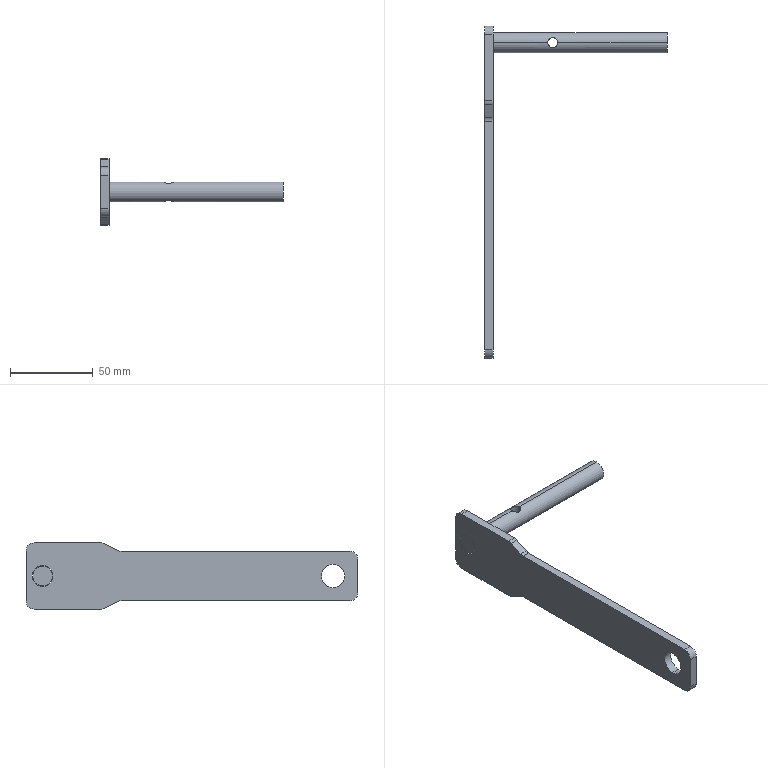Part | SolidWorks | features ICE 2, Fillet 1, Sweep 1 | 2 solids | 28 faces | box 110 x 200 x 40 mm | volume 43181 mm3 | cylinder 16 | plane 12 | commonest cylinder face diameters 10 x8 6 x2 12 x2 12.5 x2 14 x2
STEP:
#1=CARTESIAN_POINT('',(154.,-190.,-6.));
#2=VERTEX_POINT('',#1);
#3=CARTESIAN_POINT('',(148.,-190.,-6.));
#4=VERTEX_POINT('',#3);
#5=CARTESIAN_POINT('',(154.,-190.,-6.));
#6=CARTESIAN_POINT('',(154.,-190.199,-6.));
#7=CARTESIAN_POINT('',(153.98,-190.401,-5.99));
#8=CARTESIAN_POINT('',(153.901,-190.79,-5.951));
#9=CARTESIAN_POINT('',(153.843,-190.978,-5.923));
#10=CARTESIAN_POINT('',(153.689,-191.344,-5.851));
#11=CARTESIAN_POINT('',(153.596,-191.516,-5.808));
#12=CARTESIAN_POINT('',(153.38,-191.837,-5.714));
#13=CARTESIAN_POINT('',(153.255,-191.988,-5.663));
#14=CARTESIAN_POINT('',(152.982,-192.26,-5.56));
#15=CARTESIAN_POINT('',(152.834,-192.382,-5.508));
#16=CARTESIAN_POINT('',(152.512,-192.598,-5.409));
#17=CARTESIAN_POINT('',(152.338,-192.692,-5.363));
#18=CARTESIAN_POINT('',(151.98,-192.842,-5.285));
#19=CARTESIAN_POINT('',(151.793,-192.9,-5.253));
#20=CARTESIAN_POINT('',(151.401,-192.98,-5.208));
#21=CARTESIAN_POINT('',(151.202,-193.,-5.196));
#22=CARTESIAN_POINT('',(150.805,-193.,-5.196));
#23=CARTESIAN_POINT('',(150.604,-192.98,-5.208));
#24=CARTESIAN_POINT('',(150.213,-192.902,-5.252));
#25=CARTESIAN_POINT('',(150.025,-192.844,-5.284));
#26=CARTESIAN_POINT('',(149.481,-192.617,-5.402));
#27=CARTESIAN_POINT('',(149.155,-192.397,-5.508));
#28=CARTESIAN_POINT('',(148.744,-191.987,-5.663));
#29=CARTESIAN_POINT('',(148.621,-191.838,-5.714));
#30=CARTESIAN_POINT('',(148.405,-191.517,-5.807));
#31=CARTESIAN_POINT('',(148.31,-191.342,-5.851));
#32=CARTESIAN_POINT('',(148.158,-190.981,-5.922));
#33=CARTESIAN_POINT('',(148.1,-190.794,-5.951));
#34=CARTESIAN_POINT('',(148.021,-190.404,-5.99));
#35=CARTESIAN_POINT('',(148.,-190.202,-6.));
#36=CARTESIAN_POINT('',(148.,-190.,-6.));
#37=B_SPLINE_CURVE_WITH_KNOTS('',3,(#5,#6,#7,#8,#9,#10,#11,#12,#13,#14,#15,#16,#17,#18,#19,#20,#21,#22,#23,#24,#25,#26,#27,#28,#29,#30,#31,#32,#33,#34,#35,#36),.UNSPECIFIED.,.F.,.F.,(4,2,2,2,2,2,2,2,2,2,2,2,2,2,2,4),(0.009543,0.01014,0.01073,0.01133,0.01192,0.01252,0.01312,0.01371,0.01431,0.0149,0.0155,0.01669,0.01728,0.01788,0.01847,0.01907),.UNSPECIFIED.);
#38=EDGE_CURVE('',#2,#4,#37,.T.);
#39=ORIENTED_EDGE('',*,*,#38,.T.);
#40=CARTESIAN_POINT('',(148.,-190.,6.));
#41=VERTEX_POINT('',#40);
#42=CARTESIAN_POINT('',(148.,-190.,-40.));
#43=DIRECTION('',(0.,0.,1.));
#44=VECTOR('',#43,1000.);
#45=LINE('',#42,#44);
#46=EDGE_CURVE('',#4,#41,#45,.T.);
#47=ORIENTED_EDGE('',*,*,#46,.T.);
#48=CARTESIAN_POINT('',(154.,-190.,6.));
#49=VERTEX_POINT('',#48);
#50=CARTESIAN_POINT('',(148.,-190.,6.));
#51=CARTESIAN_POINT('',(148.,-190.199,6.));
#52=CARTESIAN_POINT('',(148.02,-190.401,5.99));
#53=CARTESIAN_POINT('',(148.099,-190.79,5.951));
#54=CARTESIAN_POINT('',(148.157,-190.978,5.923));
#55=CARTESIAN_POINT('',(148.311,-191.344,5.851));
#56=CARTESIAN_POINT('',(148.404,-191.516,5.808));
#57=CARTESIAN_POINT('',(148.62,-191.837,5.714));
#58=CARTESIAN_POINT('',(148.745,-191.988,5.663));
#59=CARTESIAN_POINT('',(149.018,-192.26,5.56));
#60=CARTESIAN_POINT('',(149.166,-192.382,5.508));
#61=CARTESIAN_POINT('',(149.488,-192.598,5.409));
#62=CARTESIAN_POINT('',(149.662,-192.692,5.363));
#63=CARTESIAN_POINT('',(150.02,-192.842,5.285));
#64=CARTESIAN_POINT('',(150.207,-192.9,5.253));
#65=CARTESIAN_POINT('',(150.599,-192.98,5.208));
#66=CARTESIAN_POINT('',(150.798,-193.,5.196));
#67=CARTESIAN_POINT('',(151.195,-193.,5.196));
#68=CARTESIAN_POINT('',(151.396,-192.98,5.208));
#69=CARTESIAN_POINT('',(151.787,-192.902,5.252));
#70=CARTESIAN_POINT('',(151.975,-192.844,5.284));
#71=CARTESIAN_POINT('',(152.519,-192.617,5.402));
#72=CARTESIAN_POINT('',(152.845,-192.397,5.508));
#73=CARTESIAN_POINT('',(153.256,-191.987,5.663));
#74=CARTESIAN_POINT('',(153.379,-191.838,5.714));
#75=CARTESIAN_POINT('',(153.595,-191.517,5.807));
#76=CARTESIAN_POINT('',(153.69,-191.342,5.851));
#77=CARTESIAN_POINT('',(153.842,-190.981,5.922));
#78=CARTESIAN_POINT('',(153.9,-190.794,5.951));
#79=CARTESIAN_POINT('',(153.979,-190.404,5.99));
#80=CARTESIAN_POINT('',(154.,-190.202,6.));
#81=CARTESIAN_POINT('',(154.,-190.,6.));
#82=B_SPLINE_CURVE_WITH_KNOTS('',3,(#50,#51,#52,#53,#54,#55,#56,#57,#58,#59,#60,#61,#62,#63,#64,#65,#66,#67,#68,#69,#70,#71,#72,#73,#74,#75,#76,#77,#78,#79,#80,#81),.UNSPECIFIED.,.F.,.F.,(4,2,2,2,2,2,2,2,2,2,2,2,2,2,2,4),(0.009543,0.01014,0.01073,0.01133,0.01192,0.01252,0.01312,0.01371,0.01431,0.0149,0.0155,0.01669,0.01728,0.01788,0.01847,0.01907),.UNSPECIFIED.);
#83=EDGE_CURVE('',#41,#49,#82,.T.);
#84=ORIENTED_EDGE('',*,*,#83,.T.);
#85=CARTESIAN_POINT('',(154.,-190.,-40.));
#86=DIRECTION('',(0.,0.,1.));
#87=VECTOR('',#86,1000.);
#88=LINE('',#85,#87);
#89=EDGE_CURVE('',#2,#49,#88,.T.);
#90=ORIENTED_EDGE('',*,*,#89,.F.);
#91=EDGE_LOOP('',(#39,#47,#84,#90));
#92=FACE_OUTER_BOUND('',#91,.T.);
#93=CARTESIAN_POINT('',(151.,-190.,-40.));
#94=DIRECTION('',(0.,0.,1.));
#95=DIRECTION('',(1.,0.,0.));
#96=AXIS2_PLACEMENT_3D('',#93,#94,#95);
#97=CYLINDRICAL_SURFACE('',#96,3.);
#98=ADVANCED_FACE('',(#92),#97,.F.);
#99=CARTESIAN_POINT('',(110.,-190.,-6.));
#100=VERTEX_POINT('',#99);
#101=CARTESIAN_POINT('',(110.,-190.,6.));
#102=VERTEX_POINT('',#101);
#103=CARTESIAN_POINT('',(110.,-190.,0.));
#104=DIRECTION('',(1.,0.,0.));
#105=DIRECTION('',(0.,0.,-1.));
#106=AXIS2_PLACEMENT_3D('',#103,#104,#105);
#107=CIRCLE('',#106,6.);
#108=EDGE_CURVE('',#100,#102,#107,.T.);
#109=ORIENTED_EDGE('',*,*,#108,.T.);
#110=CARTESIAN_POINT('',(110.,-190.,6.));
#111=DIRECTION('',(1.,0.,0.));
#112=VECTOR('',#111,1000.);
#113=LINE('',#110,#112);
#114=EDGE_CURVE('',#102,#41,#113,.T.);
#115=ORIENTED_EDGE('',*,*,#114,.T.);
#116=CARTESIAN_POINT('',(154.,-190.,6.));
#117=CARTESIAN_POINT('',(154.,-189.798,6.));
#118=CARTESIAN_POINT('',(153.98,-189.6,5.99));
#119=CARTESIAN_POINT('',(153.901,-189.212,5.951));
#120=CARTESIAN_POINT('',(153.842,-189.02,5.922));
#121=CARTESIAN_POINT('',(153.69,-188.657,5.851));
#122=CARTESIAN_POINT('',(153.597,-188.486,5.808));
#123=CARTESIAN_POINT('',(153.379,-188.162,5.714));
#124=CARTESIAN_POINT('',(153.255,-188.012,5.663));
#125=CARTESIAN_POINT('',(152.983,-187.74,5.56));
#126=CARTESIAN_POINT('',(152.832,-187.617,5.508));
#127=CARTESIAN_POINT('',(152.51,-187.4,5.409));
#128=CARTESIAN_POINT('',(152.339,-187.309,5.363));
#129=CARTESIAN_POINT('',(151.98,-187.158,5.285));
#130=CARTESIAN_POINT('',(151.788,-187.099,5.252));
#131=CARTESIAN_POINT('',(151.399,-187.02,5.208));
#132=CARTESIAN_POINT('',(151.203,-187.,5.196));
#133=CARTESIAN_POINT('',(150.803,-187.,5.196));
#134=CARTESIAN_POINT('',(150.601,-187.02,5.208));
#135=CARTESIAN_POINT('',(150.213,-187.098,5.252));
#136=CARTESIAN_POINT('',(150.022,-187.157,5.284));
#137=CARTESIAN_POINT('',(149.659,-187.309,5.363));
#138=CARTESIAN_POINT('',(149.488,-187.402,5.409));
#139=CARTESIAN_POINT('',(149.166,-187.618,5.508));
#140=CARTESIAN_POINT('',(149.015,-187.742,5.561));
#141=CARTESIAN_POINT('',(148.743,-188.015,5.664));
#142=CARTESIAN_POINT('',(148.62,-188.163,5.714));
#143=CARTESIAN_POINT('',(148.401,-188.488,5.809));
#144=CARTESIAN_POINT('',(148.309,-188.66,5.851));
#145=CARTESIAN_POINT('',(148.158,-189.021,5.922));
#146=CARTESIAN_POINT('',(148.099,-189.211,5.951));
#147=CARTESIAN_POINT('',(148.02,-189.603,5.99));
#148=CARTESIAN_POINT('',(148.,-189.801,6.));
#149=CARTESIAN_POINT('',(148.,-190.,6.));
#150=B_SPLINE_CURVE_WITH_KNOTS('',3,(#116,#117,#118,#119,#120,#121,#122,#123,#124,#125,#126,#127,#128,#129,#130,#131,#132,#133,#134,#135,#136,#137,#138,#139,#140,#141,#142,#143,#144,#145,#146,#147,#148,#149),.UNSPECIFIED.,.F.,.F.,(4,2,2,2,2,2,2,2,2,2,2,2,2,2,2,2,4),(0.,0.0005964,0.001193,0.001789,0.002386,0.002982,0.003579,0.004175,0.004771,0.005368,0.005964,0.006561,0.007157,0.007754,0.00835,0.008947,0.009543),.UNSPECIFIED.);
#151=EDGE_CURVE('',#49,#41,#150,.T.);
#152=ORIENTED_EDGE('',*,*,#151,.F.);
#153=CARTESIAN_POINT('',(220.,-190.,6.));
#154=VERTEX_POINT('',#153);
#155=CARTESIAN_POINT('',(110.,-190.,6.));
#156=DIRECTION('',(1.,0.,0.));
#157=VECTOR('',#156,1000.);
#158=LINE('',#155,#157);
#159=EDGE_CURVE('',#49,#154,#158,.T.);
#160=ORIENTED_EDGE('',*,*,#159,.T.);
#161=CARTESIAN_POINT('',(220.,-190.,-6.));
#162=VERTEX_POINT('',#161);
#163=CARTESIAN_POINT('',(220.,-190.,0.));
#164=DIRECTION('',(1.,0.,0.));
#165=DIRECTION('',(0.,0.,-1.));
#166=AXIS2_PLACEMENT_3D('',#163,#164,#165);
#167=CIRCLE('',#166,6.);
#168=EDGE_CURVE('',#162,#154,#167,.T.);
#169=ORIENTED_EDGE('',*,*,#168,.F.);
#170=CARTESIAN_POINT('',(110.,-190.,-6.));
#171=DIRECTION('',(1.,0.,0.));
#172=VECTOR('',#171,1000.);
#173=LINE('',#170,#172);
#174=EDGE_CURVE('',#2,#162,#173,.T.);
#175=ORIENTED_EDGE('',*,*,#174,.F.);
#176=CARTESIAN_POINT('',(148.,-190.,-6.));
#177=CARTESIAN_POINT('',(148.,-189.798,-6.));
#178=CARTESIAN_POINT('',(148.02,-189.6,-5.99));
#179=CARTESIAN_POINT('',(148.099,-189.212,-5.951));
#180=CARTESIAN_POINT('',(148.158,-189.02,-5.922));
#181=CARTESIAN_POINT('',(148.31,-188.657,-5.851));
#182=CARTESIAN_POINT('',(148.403,-188.486,-5.808));
#183=CARTESIAN_POINT('',(148.621,-188.162,-5.714));
#184=CARTESIAN_POINT('',(148.745,-188.012,-5.663));
#185=CARTESIAN_POINT('',(149.017,-187.74,-5.56));
#186=CARTESIAN_POINT('',(149.168,-187.617,-5.508));
#187=CARTESIAN_POINT('',(149.49,-187.4,-5.409));
#188=CARTESIAN_POINT('',(149.661,-187.309,-5.363));
#189=CARTESIAN_POINT('',(150.02,-187.158,-5.285));
#190=CARTESIAN_POINT('',(150.212,-187.099,-5.252));
#191=CARTESIAN_POINT('',(150.601,-187.02,-5.208));
#192=CARTESIAN_POINT('',(150.797,-187.,-5.196));
#193=CARTESIAN_POINT('',(151.197,-187.,-5.196));
#194=CARTESIAN_POINT('',(151.399,-187.02,-5.208));
#195=CARTESIAN_POINT('',(151.787,-187.098,-5.252));
#196=CARTESIAN_POINT('',(151.978,-187.157,-5.284));
#197=CARTESIAN_POINT('',(152.341,-187.309,-5.363));
#198=CARTESIAN_POINT('',(152.512,-187.402,-5.409));
#199=CARTESIAN_POINT('',(152.834,-187.618,-5.508));
#200=CARTESIAN_POINT('',(152.985,-187.742,-5.561));
#201=CARTESIAN_POINT('',(153.257,-188.015,-5.664));
#202=CARTESIAN_POINT('',(153.38,-188.163,-5.714));
#203=CARTESIAN_POINT('',(153.599,-188.488,-5.809));
#204=CARTESIAN_POINT('',(153.691,-188.66,-5.851));
#205=CARTESIAN_POINT('',(153.842,-189.021,-5.922));
#206=CARTESIAN_POINT('',(153.901,-189.211,-5.951));
#207=CARTESIAN_POINT('',(153.98,-189.603,-5.99));
#208=CARTESIAN_POINT('',(154.,-189.801,-6.));
#209=CARTESIAN_POINT('',(154.,-190.,-6.));
#210=B_SPLINE_CURVE_WITH_KNOTS('',3,(#176,#177,#178,#179,#180,#181,#182,#183,#184,#185,#186,#187,#188,#189,#190,#191,#192,#193,#194,#195,#196,#197,#198,#199,#200,#201,#202,#203,#204,#205,#206,#207,#208,#209),.UNSPECIFIED.,.F.,.F.,(4,2,2,2,2,2,2,2,2,2,2,2,2,2,2,2,4),(0.,0.0005964,0.001193,0.001789,0.002386,0.002982,0.003579,0.004175,0.004771,0.005368,0.005964,0.006561,0.007157,0.007754,0.00835,0.008947,0.009543),.UNSPECIFIED.);
#211=EDGE_CURVE('',#4,#2,#210,.T.);
#212=ORIENTED_EDGE('',*,*,#211,.F.);
#213=CARTESIAN_POINT('',(110.,-190.,-6.));
#214=DIRECTION('',(1.,0.,0.));
#215=VECTOR('',#214,1000.);
#216=LINE('',#213,#215);
#217=EDGE_CURVE('',#100,#4,#216,.T.);
#218=ORIENTED_EDGE('',*,*,#217,.F.);
#219=EDGE_LOOP('',(#109,#115,#152,#160,#169,#175,#212,#218));
#220=FACE_OUTER_BOUND('',#219,.T.);
#221=CARTESIAN_POINT('',(110.,-190.,0.));
#222=DIRECTION('',(1.,0.,0.));
#223=DIRECTION('',(0.,0.,-1.));
#224=AXIS2_PLACEMENT_3D('',#221,#222,#223);
#225=CYLINDRICAL_SURFACE('',#224,6.);
#226=ADVANCED_FACE('',(#220),#225,.T.);
#227=ORIENTED_EDGE('',*,*,#114,.F.);
#228=CARTESIAN_POINT('',(110.,-190.,0.));
#229=DIRECTION('',(1.,0.,0.));
#230=DIRECTION('',(0.,0.,-1.));
#231=AXIS2_PLACEMENT_3D('',#228,#229,#230);
#232=CIRCLE('',#231,6.);
#233=EDGE_CURVE('',#102,#100,#232,.T.);
#234=ORIENTED_EDGE('',*,*,#233,.T.);
#235=ORIENTED_EDGE('',*,*,#217,.T.);
#236=ORIENTED_EDGE('',*,*,#38,.F.);
#237=ORIENTED_EDGE('',*,*,#174,.T.);
#238=CARTESIAN_POINT('',(220.,-190.,0.));
#239=DIRECTION('',(1.,0.,0.));
#240=DIRECTION('',(0.,0.,-1.));
#241=AXIS2_PLACEMENT_3D('',#238,#239,#240);
#242=CIRCLE('',#241,6.);
#243=EDGE_CURVE('',#154,#162,#242,.T.);
#244=ORIENTED_EDGE('',*,*,#243,.F.);
#245=ORIENTED_EDGE('',*,*,#159,.F.);
#246=ORIENTED_EDGE('',*,*,#83,.F.);
#247=EDGE_LOOP('',(#227,#234,#235,#236,#237,#244,#245,#246));
#248=FACE_OUTER_BOUND('',#247,.T.);
#249=CARTESIAN_POINT('',(110.,-190.,0.));
#250=DIRECTION('',(1.,0.,0.));
#251=DIRECTION('',(0.,0.,-1.));
#252=AXIS2_PLACEMENT_3D('',#249,#250,#251);
#253=CYLINDRICAL_SURFACE('',#252,6.);
#254=ADVANCED_FACE('',(#248),#253,.T.);
#255=ORIENTED_EDGE('',*,*,#168,.T.);
#256=ORIENTED_EDGE('',*,*,#243,.T.);
#257=EDGE_LOOP('',(#255,#256));
#258=FACE_OUTER_BOUND('',#257,.T.);
#259=CARTESIAN_POINT('',(220.,-190.,0.));
#260=DIRECTION('',(1.,0.,0.));
#261=DIRECTION('',(0.,0.,-1.));
#262=AXIS2_PLACEMENT_3D('',#259,#260,#261);
#263=PLANE('',#262);
#264=ADVANCED_FACE('',(#258),#263,.T.);
#265=ORIENTED_EDGE('',*,*,#108,.F.);
#266=ORIENTED_EDGE('',*,*,#233,.F.);
#267=EDGE_LOOP('',(#265,#266));
#268=FACE_OUTER_BOUND('',#267,.T.);
#269=CARTESIAN_POINT('',(110.,-190.,0.));
#270=DIRECTION('',(1.,0.,0.));
#271=DIRECTION('',(0.,0.,-1.));
#272=AXIS2_PLACEMENT_3D('',#269,#270,#271);
#273=PLANE('',#272);
#274=ADVANCED_FACE('',(#268),#273,.F.);
#275=ORIENTED_EDGE('',*,*,#46,.F.);
#276=ORIENTED_EDGE('',*,*,#211,.T.);
#277=ORIENTED_EDGE('',*,*,#89,.T.);
#278=ORIENTED_EDGE('',*,*,#151,.T.);
#279=EDGE_LOOP('',(#275,#276,#277,#278));
#280=FACE_OUTER_BOUND('',#279,.T.);
#281=CARTESIAN_POINT('',(151.,-190.,-40.));
#282=DIRECTION('',(0.,0.,1.));
#283=DIRECTION('',(1.,0.,0.));
#284=AXIS2_PLACEMENT_3D('',#281,#282,#283);
#285=CYLINDRICAL_SURFACE('',#284,3.);
#286=ADVANCED_FACE('',(#280),#285,.F.);
#287=CLOSED_SHELL('',(#98,#226,#254,#264,#274,#286));
#288=MANIFOLD_SOLID_BREP('',#287);
#289=CARTESIAN_POINT('',(115.,-190.,-6.25));
#290=VERTEX_POINT('',#289);
#291=CARTESIAN_POINT('',(115.,-190.,6.25));
#292=VERTEX_POINT('',#291);
#293=CARTESIAN_POINT('',(115.,-190.,0.));
#294=DIRECTION('',(-1.,0.,0.));
#295=DIRECTION('',(0.,0.,1.));
#296=AXIS2_PLACEMENT_3D('',#293,#294,#295);
#297=CIRCLE('',#296,6.25);
#298=EDGE_CURVE('',#290,#292,#297,.T.);
#299=ORIENTED_EDGE('',*,*,#298,.F.);
#300=CARTESIAN_POINT('',(110.,-190.,-6.25));
#301=VERTEX_POINT('',#300);
#302=CARTESIAN_POINT('',(115.,-190.,-6.25));
#303=DIRECTION('',(-1.,0.,0.));
#304=VECTOR('',#303,1000.);
#305=LINE('',#302,#304);
#306=EDGE_CURVE('',#290,#301,#305,.T.);
#307=ORIENTED_EDGE('',*,*,#306,.T.);
#308=CARTESIAN_POINT('',(110.,-190.,6.25));
#309=VERTEX_POINT('',#308);
#310=CARTESIAN_POINT('',(110.,-190.,0.));
#311=DIRECTION('',(-1.,0.,0.));
#312=DIRECTION('',(0.,0.,1.));
#313=AXIS2_PLACEMENT_3D('',#310,#311,#312);
#314=CIRCLE('',#313,6.25);
#315=EDGE_CURVE('',#301,#309,#314,.T.);
#316=ORIENTED_EDGE('',*,*,#315,.T.);
#317=CARTESIAN_POINT('',(115.,-190.,6.25));
#318=DIRECTION('',(-1.,0.,0.));
#319=VECTOR('',#318,1000.);
#320=LINE('',#317,#319);
#321=EDGE_CURVE('',#292,#309,#320,.T.);
#322=ORIENTED_EDGE('',*,*,#321,.F.);
#323=EDGE_LOOP('',(#299,#307,#316,#322));
#324=FACE_OUTER_BOUND('',#323,.T.);
#325=CARTESIAN_POINT('',(115.,-190.,0.));
#326=DIRECTION('',(-1.,0.,0.));
#327=DIRECTION('',(0.,0.,1.));
#328=AXIS2_PLACEMENT_3D('',#325,#326,#327);
#329=CYLINDRICAL_SURFACE('',#328,6.25);
#330=ADVANCED_FACE('',(#324),#329,.F.);
#331=CARTESIAN_POINT('',(115.,-365.,-7.));
#332=VERTEX_POINT('',#331);
#333=CARTESIAN_POINT('',(115.,-365.,7.));
#334=VERTEX_POINT('',#333);
#335=CARTESIAN_POINT('',(115.,-365.,0.));
#336=DIRECTION('',(-1.,0.,0.));
#337=DIRECTION('',(0.,0.,1.));
#338=AXIS2_PLACEMENT_3D('',#335,#336,#337);
#339=CIRCLE('',#338,7.);
#340=EDGE_CURVE('',#332,#334,#339,.T.);
#341=ORIENTED_EDGE('',*,*,#340,.F.);
#342=CARTESIAN_POINT('',(110.,-365.,-7.));
#343=VERTEX_POINT('',#342);
#344=CARTESIAN_POINT('',(115.,-365.,-7.));
#345=DIRECTION('',(-1.,0.,0.));
#346=VECTOR('',#345,1000.);
#347=LINE('',#344,#346);
#348=EDGE_CURVE('',#332,#343,#347,.T.);
#349=ORIENTED_EDGE('',*,*,#348,.T.);
#350=CARTESIAN_POINT('',(110.,-365.,7.));
#351=VERTEX_POINT('',#350);
#352=CARTESIAN_POINT('',(110.,-365.,0.));
#353=DIRECTION('',(-1.,0.,0.));
#354=DIRECTION('',(0.,0.,1.));
#355=AXIS2_PLACEMENT_3D('',#352,#353,#354);
#356=CIRCLE('',#355,7.);
#357=EDGE_CURVE('',#343,#351,#356,.T.);
#358=ORIENTED_EDGE('',*,*,#357,.T.);
#359=CARTESIAN_POINT('',(115.,-365.,7.));
#360=DIRECTION('',(-1.,0.,0.));
#361=VECTOR('',#360,1000.);
#362=LINE('',#359,#361);
#363=EDGE_CURVE('',#334,#351,#362,.T.);
#364=ORIENTED_EDGE('',*,*,#363,.F.);
#365=EDGE_LOOP('',(#341,#349,#358,#364));
#366=FACE_OUTER_BOUND('',#365,.T.);
#367=CARTESIAN_POINT('',(115.,-365.,0.));
#368=DIRECTION('',(-1.,0.,0.));
#369=DIRECTION('',(0.,0.,1.));
#370=AXIS2_PLACEMENT_3D('',#367,#368,#369);
#371=CYLINDRICAL_SURFACE('',#370,7.);
#372=ADVANCED_FACE('',(#366),#371,.F.);
#373=CARTESIAN_POINT('',(110.,-227.236,19.472));
#374=VERTEX_POINT('',#373);
#375=CARTESIAN_POINT('',(110.,-225.,20.));
#376=VERTEX_POINT('',#375);
#377=CARTESIAN_POINT('',(110.,-225.,15.));
#378=DIRECTION('',(-1.,0.,0.));
#379=DIRECTION('',(0.,0.,1.));
#380=AXIS2_PLACEMENT_3D('',#377,#378,#379);
#381=CIRCLE('',#380,5.);
#382=EDGE_CURVE('',#374,#376,#381,.T.);
#383=ORIENTED_EDGE('',*,*,#382,.F.);
#384=CARTESIAN_POINT('',(115.,-227.236,19.472));
#385=VERTEX_POINT('',#384);
#386=CARTESIAN_POINT('',(115.,-227.236,19.472));
#387=DIRECTION('',(-1.,0.,0.));
#388=VECTOR('',#387,1000.);
#389=LINE('',#386,#388);
#390=EDGE_CURVE('',#385,#374,#389,.T.);
#391=ORIENTED_EDGE('',*,*,#390,.F.);
#392=CARTESIAN_POINT('',(115.,-225.,20.));
#393=VERTEX_POINT('',#392);
#394=CARTESIAN_POINT('',(115.,-225.,15.));
#395=DIRECTION('',(-1.,0.,0.));
#396=DIRECTION('',(0.,0.,1.));
#397=AXIS2_PLACEMENT_3D('',#394,#395,#396);
#398=CIRCLE('',#397,5.);
#399=EDGE_CURVE('',#385,#393,#398,.T.);
#400=ORIENTED_EDGE('',*,*,#399,.T.);
#401=CARTESIAN_POINT('',(115.,-225.,20.));
#402=DIRECTION('',(-1.,0.,0.));
#403=VECTOR('',#402,1000.);
#404=LINE('',#401,#403);
#405=EDGE_CURVE('',#393,#376,#404,.T.);
#406=ORIENTED_EDGE('',*,*,#405,.T.);
#407=EDGE_LOOP('',(#383,#391,#400,#406));
#408=FACE_OUTER_BOUND('',#407,.T.);
#409=CARTESIAN_POINT('',(115.,-225.,15.));
#410=DIRECTION('',(-1.,0.,0.));
#411=DIRECTION('',(0.,0.,1.));
#412=AXIS2_PLACEMENT_3D('',#409,#410,#411);
#413=CYLINDRICAL_SURFACE('',#412,5.);
#414=ADVANCED_FACE('',(#408),#413,.T.);
#415=CARTESIAN_POINT('',(110.,-235.125,15.528));
#416=VERTEX_POINT('',#415);
#417=CARTESIAN_POINT('',(110.,-227.236,19.472));
#418=DIRECTION('',(0.,0.8944,0.4472));
#419=VECTOR('',#418,1000.);
#420=LINE('',#417,#419);
#421=EDGE_CURVE('',#416,#374,#420,.T.);
#422=ORIENTED_EDGE('',*,*,#421,.F.);
#423=CARTESIAN_POINT('',(115.,-235.125,15.528));
#424=VERTEX_POINT('',#423);
#425=CARTESIAN_POINT('',(115.,-235.125,15.528));
#426=DIRECTION('',(-1.,0.,0.));
#427=VECTOR('',#426,1000.);
#428=LINE('',#425,#427);
#429=EDGE_CURVE('',#424,#416,#428,.T.);
#430=ORIENTED_EDGE('',*,*,#429,.F.);
#431=CARTESIAN_POINT('',(115.,-227.236,19.472));
#432=DIRECTION('',(0.,0.8944,0.4472));
#433=VECTOR('',#432,1000.);
#434=LINE('',#431,#433);
#435=EDGE_CURVE('',#424,#385,#434,.T.);
#436=ORIENTED_EDGE('',*,*,#435,.T.);
#437=ORIENTED_EDGE('',*,*,#390,.T.);
#438=EDGE_LOOP('',(#422,#430,#436,#437));
#439=FACE_OUTER_BOUND('',#438,.T.);
#440=CARTESIAN_POINT('',(115.,-227.236,19.472));
#441=DIRECTION('',(0.,-0.4472,0.8944));
#442=DIRECTION('',(0.,-0.8944,-0.4472));
#443=AXIS2_PLACEMENT_3D('',#440,#441,#442);
#444=PLANE('',#443);
#445=ADVANCED_FACE('',(#439),#444,.T.);
#446=CARTESIAN_POINT('',(110.,-237.361,15.));
#447=VERTEX_POINT('',#446);
#448=CARTESIAN_POINT('',(110.,-237.361,20.));
#449=DIRECTION('',(1.,0.,0.));
#450=DIRECTION('',(0.,0.,1.));
#451=AXIS2_PLACEMENT_3D('',#448,#449,#450);
#452=CIRCLE('',#451,5.);
#453=EDGE_CURVE('',#447,#416,#452,.T.);
#454=ORIENTED_EDGE('',*,*,#453,.F.);
#455=CARTESIAN_POINT('',(115.,-237.361,15.));
#456=VERTEX_POINT('',#455);
#457=CARTESIAN_POINT('',(115.,-237.361,15.));
#458=DIRECTION('',(-1.,0.,0.));
#459=VECTOR('',#458,1000.);
#460=LINE('',#457,#459);
#461=EDGE_CURVE('',#456,#447,#460,.T.);
#462=ORIENTED_EDGE('',*,*,#461,.F.);
#463=CARTESIAN_POINT('',(115.,-237.361,20.));
#464=DIRECTION('',(1.,0.,0.));
#465=DIRECTION('',(0.,0.,1.));
#466=AXIS2_PLACEMENT_3D('',#463,#464,#465);
#467=CIRCLE('',#466,5.);
#468=EDGE_CURVE('',#456,#424,#467,.T.);
#469=ORIENTED_EDGE('',*,*,#468,.T.);
#470=ORIENTED_EDGE('',*,*,#429,.T.);
#471=EDGE_LOOP('',(#454,#462,#469,#470));
#472=FACE_OUTER_BOUND('',#471,.T.);
#473=CARTESIAN_POINT('',(115.,-237.361,20.));
#474=DIRECTION('',(-1.,0.,0.));
#475=DIRECTION('',(0.,0.,1.));
#476=AXIS2_PLACEMENT_3D('',#473,#474,#475);
#477=CYLINDRICAL_SURFACE('',#476,5.);
#478=ADVANCED_FACE('',(#472),#477,.F.);
#479=CARTESIAN_POINT('',(110.,-375.,15.));
#480=VERTEX_POINT('',#479);
#481=CARTESIAN_POINT('',(110.,-237.361,15.));
#482=DIRECTION('',(0.,1.,0.));
#483=VECTOR('',#482,1000.);
#484=LINE('',#481,#483);
#485=EDGE_CURVE('',#480,#447,#484,.T.);
#486=ORIENTED_EDGE('',*,*,#485,.F.);
#487=CARTESIAN_POINT('',(115.,-375.,15.));
#488=VERTEX_POINT('',#487);
#489=CARTESIAN_POINT('',(115.,-375.,15.));
#490=DIRECTION('',(1.,0.,0.));
#491=VECTOR('',#490,1000.);
#492=LINE('',#489,#491);
#493=EDGE_CURVE('',#480,#488,#492,.T.);
#494=ORIENTED_EDGE('',*,*,#493,.T.);
#495=CARTESIAN_POINT('',(115.,-237.361,15.));
#496=DIRECTION('',(0.,1.,0.));
#497=VECTOR('',#496,1000.);
#498=LINE('',#495,#497);
#499=EDGE_CURVE('',#488,#456,#498,.T.);
#500=ORIENTED_EDGE('',*,*,#499,.T.);
#501=ORIENTED_EDGE('',*,*,#461,.T.);
#502=EDGE_LOOP('',(#486,#494,#500,#501));
#503=FACE_OUTER_BOUND('',#502,.T.);
#504=CARTESIAN_POINT('',(115.,-237.361,15.));
#505=DIRECTION('',(0.,0.,1.));
#506=DIRECTION('',(0.,-1.,0.));
#507=AXIS2_PLACEMENT_3D('',#504,#505,#506);
#508=PLANE('',#507);
#509=ADVANCED_FACE('',(#503),#508,.T.);
#510=CARTESIAN_POINT('',(110.,-380.,-10.));
#511=VERTEX_POINT('',#510);
#512=CARTESIAN_POINT('',(110.,-380.,10.));
#513=VERTEX_POINT('',#512);
#514=CARTESIAN_POINT('',(110.,-380.,-15.));
#515=DIRECTION('',(0.,0.,1.));
#516=VECTOR('',#515,1000.);
#517=LINE('',#514,#516);
#518=EDGE_CURVE('',#511,#513,#517,.T.);
#519=ORIENTED_EDGE('',*,*,#518,.F.);
#520=CARTESIAN_POINT('',(115.,-380.,-10.));
#521=VERTEX_POINT('',#520);
#522=CARTESIAN_POINT('',(115.,-380.,-10.));
#523=DIRECTION('',(1.,0.,0.));
#524=VECTOR('',#523,1000.);
#525=LINE('',#522,#524);
#526=EDGE_CURVE('',#511,#521,#525,.T.);
#527=ORIENTED_EDGE('',*,*,#526,.T.);
#528=CARTESIAN_POINT('',(115.,-380.,10.));
#529=VERTEX_POINT('',#528);
#530=CARTESIAN_POINT('',(115.,-380.,-15.));
#531=DIRECTION('',(0.,0.,1.));
#532=VECTOR('',#531,1000.);
#533=LINE('',#530,#532);
#534=EDGE_CURVE('',#521,#529,#533,.T.);
#535=ORIENTED_EDGE('',*,*,#534,.T.);
#536=CARTESIAN_POINT('',(115.,-380.,10.));
#537=DIRECTION('',(-1.,0.,0.));
#538=VECTOR('',#537,1000.);
#539=LINE('',#536,#538);
#540=EDGE_CURVE('',#529,#513,#539,.T.);
#541=ORIENTED_EDGE('',*,*,#540,.T.);
#542=EDGE_LOOP('',(#519,#527,#535,#541));
#543=FACE_OUTER_BOUND('',#542,.T.);
#544=CARTESIAN_POINT('',(115.,-380.,-15.));
#545=DIRECTION('',(0.,-1.,0.));
#546=DIRECTION('',(0.,0.,-1.));
#547=AXIS2_PLACEMENT_3D('',#544,#545,#546);
#548=PLANE('',#547);
#549=ADVANCED_FACE('',(#543),#548,.T.);
#550=CARTESIAN_POINT('',(115.,-237.361,-15.));
#551=VERTEX_POINT('',#550);
#552=CARTESIAN_POINT('',(115.,-375.,-15.));
#553=VERTEX_POINT('',#552);
#554=CARTESIAN_POINT('',(115.,-237.361,-15.));
#555=DIRECTION('',(0.,-1.,0.));
#556=VECTOR('',#555,1000.);
#557=LINE('',#554,#556);
#558=EDGE_CURVE('',#551,#553,#557,.T.);
#559=ORIENTED_EDGE('',*,*,#558,.T.);
#560=CARTESIAN_POINT('',(110.,-375.,-15.));
#561=VERTEX_POINT('',#560);
#562=CARTESIAN_POINT('',(115.,-375.,-15.));
#563=DIRECTION('',(-1.,0.,0.));
#564=VECTOR('',#563,1000.);
#565=LINE('',#562,#564);
#566=EDGE_CURVE('',#553,#561,#565,.T.);
#567=ORIENTED_EDGE('',*,*,#566,.T.);
#568=CARTESIAN_POINT('',(110.,-237.361,-15.));
#569=VERTEX_POINT('',#568);
#570=CARTESIAN_POINT('',(110.,-237.361,-15.));
#571=DIRECTION('',(0.,-1.,0.));
#572=VECTOR('',#571,1000.);
#573=LINE('',#570,#572);
#574=EDGE_CURVE('',#569,#561,#573,.T.);
#575=ORIENTED_EDGE('',*,*,#574,.F.);
#576=CARTESIAN_POINT('',(115.,-237.361,-15.));
#577=DIRECTION('',(-1.,0.,0.));
#578=VECTOR('',#577,1000.);
#579=LINE('',#576,#578);
#580=EDGE_CURVE('',#551,#569,#579,.T.);
#581=ORIENTED_EDGE('',*,*,#580,.F.);
#582=EDGE_LOOP('',(#559,#567,#575,#581));
#583=FACE_OUTER_BOUND('',#582,.T.);
#584=CARTESIAN_POINT('',(115.,-237.361,-15.));
#585=DIRECTION('',(0.,0.,-1.));
#586=DIRECTION('',(0.,1.,0.));
#587=AXIS2_PLACEMENT_3D('',#584,#585,#586);
#588=PLANE('',#587);
#589=ADVANCED_FACE('',(#583),#588,.T.);
#590=CARTESIAN_POINT('',(110.,-235.125,-15.528));
#591=VERTEX_POINT('',#590);
#592=CARTESIAN_POINT('',(110.,-237.361,-20.));
#593=DIRECTION('',(1.,0.,0.));
#594=DIRECTION('',(0.,0.,-1.));
#595=AXIS2_PLACEMENT_3D('',#592,#593,#594);
#596=CIRCLE('',#595,5.);
#597=EDGE_CURVE('',#591,#569,#596,.T.);
#598=ORIENTED_EDGE('',*,*,#597,.F.);
#599=CARTESIAN_POINT('',(115.,-235.125,-15.528));
#600=VERTEX_POINT('',#599);
#601=CARTESIAN_POINT('',(115.,-235.125,-15.528));
#602=DIRECTION('',(-1.,0.,0.));
#603=VECTOR('',#602,1000.);
#604=LINE('',#601,#603);
#605=EDGE_CURVE('',#600,#591,#604,.T.);
#606=ORIENTED_EDGE('',*,*,#605,.F.);
#607=CARTESIAN_POINT('',(115.,-237.361,-20.));
#608=DIRECTION('',(1.,0.,0.));
#609=DIRECTION('',(0.,0.,-1.));
#610=AXIS2_PLACEMENT_3D('',#607,#608,#609);
#611=CIRCLE('',#610,5.);
#612=EDGE_CURVE('',#600,#551,#611,.T.);
#613=ORIENTED_EDGE('',*,*,#612,.T.);
#614=ORIENTED_EDGE('',*,*,#580,.T.);
#615=EDGE_LOOP('',(#598,#606,#613,#614));
#616=FACE_OUTER_BOUND('',#615,.T.);
#617=CARTESIAN_POINT('',(115.,-237.361,-20.));
#618=DIRECTION('',(-1.,0.,0.));
#619=DIRECTION('',(0.,0.,1.));
#620=AXIS2_PLACEMENT_3D('',#617,#618,#619);
#621=CYLINDRICAL_SURFACE('',#620,5.);
#622=ADVANCED_FACE('',(#616),#621,.F.);
#623=CARTESIAN_POINT('',(110.,-227.236,-19.472));
#624=VERTEX_POINT('',#623);
#625=CARTESIAN_POINT('',(110.,-227.236,-19.472));
#626=DIRECTION('',(0.,-0.8944,0.4472));
#627=VECTOR('',#626,1000.);
#628=LINE('',#625,#627);
#629=EDGE_CURVE('',#624,#591,#628,.T.);
#630=ORIENTED_EDGE('',*,*,#629,.F.);
#631=CARTESIAN_POINT('',(115.,-227.236,-19.472));
#632=VERTEX_POINT('',#631);
#633=CARTESIAN_POINT('',(115.,-227.236,-19.472));
#634=DIRECTION('',(-1.,0.,0.));
#635=VECTOR('',#634,1000.);
#636=LINE('',#633,#635);
#637=EDGE_CURVE('',#632,#624,#636,.T.);
#638=ORIENTED_EDGE('',*,*,#637,.F.);
#639=CARTESIAN_POINT('',(115.,-227.236,-19.472));
#640=DIRECTION('',(0.,-0.8944,0.4472));
#641=VECTOR('',#640,1000.);
#642=LINE('',#639,#641);
#643=EDGE_CURVE('',#632,#600,#642,.T.);
#644=ORIENTED_EDGE('',*,*,#643,.T.);
#645=ORIENTED_EDGE('',*,*,#605,.T.);
#646=EDGE_LOOP('',(#630,#638,#644,#645));
#647=FACE_OUTER_BOUND('',#646,.T.);
#648=CARTESIAN_POINT('',(115.,-227.236,-19.472));
#649=DIRECTION('',(0.,-0.4472,-0.8944));
#650=DIRECTION('',(0.,0.8944,-0.4472));
#651=AXIS2_PLACEMENT_3D('',#648,#649,#650);
#652=PLANE('',#651);
#653=ADVANCED_FACE('',(#647),#652,.T.);
#654=CARTESIAN_POINT('',(110.,-225.,-20.));
#655=VERTEX_POINT('',#654);
#656=CARTESIAN_POINT('',(110.,-225.,-15.));
#657=DIRECTION('',(-1.,0.,0.));
#658=DIRECTION('',(0.,0.,-1.));
#659=AXIS2_PLACEMENT_3D('',#656,#657,#658);
#660=CIRCLE('',#659,5.);
#661=EDGE_CURVE('',#655,#624,#660,.T.);
#662=ORIENTED_EDGE('',*,*,#661,.F.);
#663=CARTESIAN_POINT('',(115.,-225.,-20.));
#664=VERTEX_POINT('',#663);
#665=CARTESIAN_POINT('',(115.,-225.,-20.));
#666=DIRECTION('',(-1.,0.,0.));
#667=VECTOR('',#666,1000.);
#668=LINE('',#665,#667);
#669=EDGE_CURVE('',#664,#655,#668,.T.);
#670=ORIENTED_EDGE('',*,*,#669,.F.);
#671=CARTESIAN_POINT('',(115.,-225.,-15.));
#672=DIRECTION('',(-1.,0.,0.));
#673=DIRECTION('',(0.,0.,-1.));
#674=AXIS2_PLACEMENT_3D('',#671,#672,#673);
#675=CIRCLE('',#674,5.);
#676=EDGE_CURVE('',#664,#632,#675,.T.);
#677=ORIENTED_EDGE('',*,*,#676,.T.);
#678=ORIENTED_EDGE('',*,*,#637,.T.);
#679=EDGE_LOOP('',(#662,#670,#677,#678));
#680=FACE_OUTER_BOUND('',#679,.T.);
#681=CARTESIAN_POINT('',(115.,-225.,-15.));
#682=DIRECTION('',(-1.,0.,0.));
#683=DIRECTION('',(0.,0.,1.));
#684=AXIS2_PLACEMENT_3D('',#681,#682,#683);
#685=CYLINDRICAL_SURFACE('',#684,5.);
#686=ADVANCED_FACE('',(#680),#685,.T.);
#687=CARTESIAN_POINT('',(110.,-185.,-20.));
#688=VERTEX_POINT('',#687);
#689=CARTESIAN_POINT('',(110.,-185.,-20.));
#690=DIRECTION('',(0.,-1.,0.));
#691=VECTOR('',#690,1000.);
#692=LINE('',#689,#691);
#693=EDGE_CURVE('',#688,#655,#692,.T.);
#694=ORIENTED_EDGE('',*,*,#693,.F.);
#695=CARTESIAN_POINT('',(115.,-185.,-20.));
#696=VERTEX_POINT('',#695);
#697=CARTESIAN_POINT('',(115.,-185.,-20.));
#698=DIRECTION('',(-1.,0.,0.));
#699=VECTOR('',#698,1000.);
#700=LINE('',#697,#699);
#701=EDGE_CURVE('',#696,#688,#700,.T.);
#702=ORIENTED_EDGE('',*,*,#701,.F.);
#703=CARTESIAN_POINT('',(115.,-185.,-20.));
#704=DIRECTION('',(0.,-1.,0.));
#705=VECTOR('',#704,1000.);
#706=LINE('',#703,#705);
#707=EDGE_CURVE('',#696,#664,#706,.T.);
#708=ORIENTED_EDGE('',*,*,#707,.T.);
#709=ORIENTED_EDGE('',*,*,#669,.T.);
#710=EDGE_LOOP('',(#694,#702,#708,#709));
#711=FACE_OUTER_BOUND('',#710,.T.);
#712=CARTESIAN_POINT('',(115.,-185.,-20.));
#713=DIRECTION('',(0.,0.,-1.));
#714=DIRECTION('',(0.,1.,0.));
#715=AXIS2_PLACEMENT_3D('',#712,#713,#714);
#716=PLANE('',#715);
#717=ADVANCED_FACE('',(#711),#716,.T.);
#718=CARTESIAN_POINT('',(110.,-180.,-15.));
#719=VERTEX_POINT('',#718);
#720=CARTESIAN_POINT('',(110.,-185.,-15.));
#721=DIRECTION('',(-1.,0.,0.));
#722=DIRECTION('',(0.,0.,1.));
#723=AXIS2_PLACEMENT_3D('',#720,#721,#722);
#724=CIRCLE('',#723,5.);
#725=EDGE_CURVE('',#719,#688,#724,.T.);
#726=ORIENTED_EDGE('',*,*,#725,.F.);
#727=CARTESIAN_POINT('',(115.,-180.,-15.));
#728=VERTEX_POINT('',#727);
#729=CARTESIAN_POINT('',(115.,-180.,-15.));
#730=DIRECTION('',(-1.,0.,0.));
#731=VECTOR('',#730,1000.);
#732=LINE('',#729,#731);
#733=EDGE_CURVE('',#728,#719,#732,.T.);
#734=ORIENTED_EDGE('',*,*,#733,.F.);
#735=CARTESIAN_POINT('',(115.,-185.,-15.));
#736=DIRECTION('',(-1.,0.,0.));
#737=DIRECTION('',(0.,0.,1.));
#738=AXIS2_PLACEMENT_3D('',#735,#736,#737);
#739=CIRCLE('',#738,5.);
#740=EDGE_CURVE('',#728,#696,#739,.T.);
#741=ORIENTED_EDGE('',*,*,#740,.T.);
#742=ORIENTED_EDGE('',*,*,#701,.T.);
#743=EDGE_LOOP('',(#726,#734,#741,#742));
#744=FACE_OUTER_BOUND('',#743,.T.);
#745=CARTESIAN_POINT('',(115.,-185.,-15.));
#746=DIRECTION('',(-1.,0.,0.));
#747=DIRECTION('',(0.,0.,1.));
#748=AXIS2_PLACEMENT_3D('',#745,#746,#747);
#749=CYLINDRICAL_SURFACE('',#748,5.);
#750=ADVANCED_FACE('',(#744),#749,.T.);
#751=CARTESIAN_POINT('',(110.,-180.,15.));
#752=VERTEX_POINT('',#751);
#753=CARTESIAN_POINT('',(110.,-180.,-15.));
#754=DIRECTION('',(0.,0.,-1.));
#755=VECTOR('',#754,1000.);
#756=LINE('',#753,#755);
#757=EDGE_CURVE('',#752,#719,#756,.T.);
#758=ORIENTED_EDGE('',*,*,#757,.F.);
#759=CARTESIAN_POINT('',(115.,-180.,15.));
#760=VERTEX_POINT('',#759);
#761=CARTESIAN_POINT('',(115.,-180.,15.));
#762=DIRECTION('',(-1.,0.,0.));
#763=VECTOR('',#762,1000.);
#764=LINE('',#761,#763);
#765=EDGE_CURVE('',#760,#752,#764,.T.);
#766=ORIENTED_EDGE('',*,*,#765,.F.);
#767=CARTESIAN_POINT('',(115.,-180.,-15.));
#768=DIRECTION('',(0.,0.,-1.));
#769=VECTOR('',#768,1000.);
#770=LINE('',#767,#769);
#771=EDGE_CURVE('',#760,#728,#770,.T.);
#772=ORIENTED_EDGE('',*,*,#771,.T.);
#773=ORIENTED_EDGE('',*,*,#733,.T.);
#774=EDGE_LOOP('',(#758,#766,#772,#773));
#775=FACE_OUTER_BOUND('',#774,.T.);
#776=CARTESIAN_POINT('',(115.,-180.,-15.));
#777=DIRECTION('',(0.,1.,0.));
#778=DIRECTION('',(0.,0.,1.));
#779=AXIS2_PLACEMENT_3D('',#776,#777,#778);
#780=PLANE('',#779);
#781=ADVANCED_FACE('',(#775),#780,.T.);
#782=CARTESIAN_POINT('',(110.,-185.,20.));
#783=VERTEX_POINT('',#782);
#784=CARTESIAN_POINT('',(110.,-185.,15.));
#785=DIRECTION('',(-1.,0.,0.));
#786=DIRECTION('',(0.,0.,-1.));
#787=AXIS2_PLACEMENT_3D('',#784,#785,#786);
#788=CIRCLE('',#787,5.);
#789=EDGE_CURVE('',#783,#752,#788,.T.);
#790=ORIENTED_EDGE('',*,*,#789,.F.);
#791=CARTESIAN_POINT('',(115.,-185.,20.));
#792=VERTEX_POINT('',#791);
#793=CARTESIAN_POINT('',(115.,-185.,20.));
#794=DIRECTION('',(-1.,0.,0.));
#795=VECTOR('',#794,1000.);
#796=LINE('',#793,#795);
#797=EDGE_CURVE('',#792,#783,#796,.T.);
#798=ORIENTED_EDGE('',*,*,#797,.F.);
#799=CARTESIAN_POINT('',(115.,-185.,15.));
#800=DIRECTION('',(-1.,0.,0.));
#801=DIRECTION('',(0.,0.,-1.));
#802=AXIS2_PLACEMENT_3D('',#799,#800,#801);
#803=CIRCLE('',#802,5.);
#804=EDGE_CURVE('',#792,#760,#803,.T.);
#805=ORIENTED_EDGE('',*,*,#804,.T.);
#806=ORIENTED_EDGE('',*,*,#765,.T.);
#807=EDGE_LOOP('',(#790,#798,#805,#806));
#808=FACE_OUTER_BOUND('',#807,.T.);
#809=CARTESIAN_POINT('',(115.,-185.,15.));
#810=DIRECTION('',(-1.,0.,0.));
#811=DIRECTION('',(0.,0.,1.));
#812=AXIS2_PLACEMENT_3D('',#809,#810,#811);
#813=CYLINDRICAL_SURFACE('',#812,5.);
#814=ADVANCED_FACE('',(#808),#813,.T.);
#815=CARTESIAN_POINT('',(110.,-185.,20.));
#816=DIRECTION('',(0.,1.,0.));
#817=VECTOR('',#816,1000.);
#818=LINE('',#815,#817);
#819=EDGE_CURVE('',#376,#783,#818,.T.);
#820=ORIENTED_EDGE('',*,*,#819,.F.);
#821=ORIENTED_EDGE('',*,*,#405,.F.);
#822=CARTESIAN_POINT('',(115.,-185.,20.));
#823=DIRECTION('',(0.,1.,0.));
#824=VECTOR('',#823,1000.);
#825=LINE('',#822,#824);
#826=EDGE_CURVE('',#393,#792,#825,.T.);
#827=ORIENTED_EDGE('',*,*,#826,.T.);
#828=ORIENTED_EDGE('',*,*,#797,.T.);
#829=EDGE_LOOP('',(#820,#821,#827,#828));
#830=FACE_OUTER_BOUND('',#829,.T.);
#831=CARTESIAN_POINT('',(115.,-185.,20.));
#832=DIRECTION('',(0.,0.,1.));
#833=DIRECTION('',(0.,-1.,0.));
#834=AXIS2_PLACEMENT_3D('',#831,#832,#833);
#835=PLANE('',#834);
#836=ADVANCED_FACE('',(#830),#835,.T.);
#837=CARTESIAN_POINT('',(115.,-190.,0.));
#838=DIRECTION('',(-1.,0.,0.));
#839=DIRECTION('',(0.,0.,1.));
#840=AXIS2_PLACEMENT_3D('',#837,#838,#839);
#841=CIRCLE('',#840,6.25);
#842=EDGE_CURVE('',#292,#290,#841,.T.);
#843=ORIENTED_EDGE('',*,*,#842,.T.);
#844=ORIENTED_EDGE('',*,*,#298,.T.);
#845=EDGE_LOOP('',(#843,#844));
#846=FACE_BOUND('',#845,.T.);
#847=CARTESIAN_POINT('',(115.,-365.,0.));
#848=DIRECTION('',(-1.,0.,0.));
#849=DIRECTION('',(0.,0.,1.));
#850=AXIS2_PLACEMENT_3D('',#847,#848,#849);
#851=CIRCLE('',#850,7.);
#852=EDGE_CURVE('',#334,#332,#851,.T.);
#853=ORIENTED_EDGE('',*,*,#852,.T.);
#854=ORIENTED_EDGE('',*,*,#340,.T.);
#855=EDGE_LOOP('',(#853,#854));
#856=FACE_BOUND('',#855,.T.);
#857=ORIENTED_EDGE('',*,*,#534,.F.);
#858=CARTESIAN_POINT('',(115.,-375.,-10.));
#859=DIRECTION('',(1.,0.,0.));
#860=DIRECTION('',(0.,0.,1.));
#861=AXIS2_PLACEMENT_3D('',#858,#859,#860);
#862=CIRCLE('',#861,5.);
#863=EDGE_CURVE('',#521,#553,#862,.T.);
#864=ORIENTED_EDGE('',*,*,#863,.T.);
#865=ORIENTED_EDGE('',*,*,#558,.F.);
#866=ORIENTED_EDGE('',*,*,#612,.F.);
#867=ORIENTED_EDGE('',*,*,#643,.F.);
#868=ORIENTED_EDGE('',*,*,#676,.F.);
#869=ORIENTED_EDGE('',*,*,#707,.F.);
#870=ORIENTED_EDGE('',*,*,#740,.F.);
#871=ORIENTED_EDGE('',*,*,#771,.F.);
#872=ORIENTED_EDGE('',*,*,#804,.F.);
#873=ORIENTED_EDGE('',*,*,#826,.F.);
#874=ORIENTED_EDGE('',*,*,#399,.F.);
#875=ORIENTED_EDGE('',*,*,#435,.F.);
#876=ORIENTED_EDGE('',*,*,#468,.F.);
#877=ORIENTED_EDGE('',*,*,#499,.F.);
#878=CARTESIAN_POINT('',(115.,-375.,10.));
#879=DIRECTION('',(1.,0.,0.));
#880=DIRECTION('',(0.,0.,1.));
#881=AXIS2_PLACEMENT_3D('',#878,#879,#880);
#882=CIRCLE('',#881,5.);
#883=EDGE_CURVE('',#488,#529,#882,.T.);
#884=ORIENTED_EDGE('',*,*,#883,.T.);
#885=EDGE_LOOP('',(#857,#864,#865,#866,#867,#868,#869,#870,#871,#872,#873,#874,#875,#876,#877,#884));
#886=FACE_OUTER_BOUND('',#885,.T.);
#887=CARTESIAN_POINT('',(115.,-225.,15.));
#888=DIRECTION('',(-1.,0.,0.));
#889=DIRECTION('',(0.,0.,1.));
#890=AXIS2_PLACEMENT_3D('',#887,#888,#889);
#891=PLANE('',#890);
#892=ADVANCED_FACE('',(#846,#856,#886),#891,.F.);
#893=CARTESIAN_POINT('',(110.,-190.,0.));
#894=DIRECTION('',(-1.,0.,0.));
#895=DIRECTION('',(0.,0.,1.));
#896=AXIS2_PLACEMENT_3D('',#893,#894,#895);
#897=CIRCLE('',#896,6.25);
#898=EDGE_CURVE('',#309,#301,#897,.T.);
#899=ORIENTED_EDGE('',*,*,#898,.F.);
#900=ORIENTED_EDGE('',*,*,#315,.F.);
#901=EDGE_LOOP('',(#899,#900));
#902=FACE_BOUND('',#901,.T.);
#903=CARTESIAN_POINT('',(110.,-365.,0.));
#904=DIRECTION('',(-1.,0.,0.));
#905=DIRECTION('',(0.,0.,1.));
#906=AXIS2_PLACEMENT_3D('',#903,#904,#905);
#907=CIRCLE('',#906,7.);
#908=EDGE_CURVE('',#351,#343,#907,.T.);
#909=ORIENTED_EDGE('',*,*,#908,.F.);
#910=ORIENTED_EDGE('',*,*,#357,.F.);
#911=EDGE_LOOP('',(#909,#910));
#912=FACE_BOUND('',#911,.T.);
#913=ORIENTED_EDGE('',*,*,#574,.T.);
#914=CARTESIAN_POINT('',(110.,-375.,-10.));
#915=DIRECTION('',(-1.,0.,0.));
#916=DIRECTION('',(0.,0.,1.));
#917=AXIS2_PLACEMENT_3D('',#914,#915,#916);
#918=CIRCLE('',#917,5.);
#919=EDGE_CURVE('',#561,#511,#918,.T.);
#920=ORIENTED_EDGE('',*,*,#919,.T.);
#921=ORIENTED_EDGE('',*,*,#518,.T.);
#922=CARTESIAN_POINT('',(110.,-375.,10.));
#923=DIRECTION('',(-1.,0.,0.));
#924=DIRECTION('',(0.,0.,1.));
#925=AXIS2_PLACEMENT_3D('',#922,#923,#924);
#926=CIRCLE('',#925,5.);
#927=EDGE_CURVE('',#513,#480,#926,.T.);
#928=ORIENTED_EDGE('',*,*,#927,.T.);
#929=ORIENTED_EDGE('',*,*,#485,.T.);
#930=ORIENTED_EDGE('',*,*,#453,.T.);
#931=ORIENTED_EDGE('',*,*,#421,.T.);
#932=ORIENTED_EDGE('',*,*,#382,.T.);
#933=ORIENTED_EDGE('',*,*,#819,.T.);
#934=ORIENTED_EDGE('',*,*,#789,.T.);
#935=ORIENTED_EDGE('',*,*,#757,.T.);
#936=ORIENTED_EDGE('',*,*,#725,.T.);
#937=ORIENTED_EDGE('',*,*,#693,.T.);
#938=ORIENTED_EDGE('',*,*,#661,.T.);
#939=ORIENTED_EDGE('',*,*,#629,.T.);
#940=ORIENTED_EDGE('',*,*,#597,.T.);
#941=EDGE_LOOP('',(#913,#920,#921,#928,#929,#930,#931,#932,#933,#934,#935,#936,#937,#938,#939,#940));
#942=FACE_OUTER_BOUND('',#941,.T.);
#943=CARTESIAN_POINT('',(110.,-225.,15.));
#944=DIRECTION('',(-1.,0.,0.));
#945=DIRECTION('',(0.,0.,1.));
#946=AXIS2_PLACEMENT_3D('',#943,#944,#945);
#947=PLANE('',#946);
#948=ADVANCED_FACE('',(#902,#912,#942),#947,.T.);
#949=ORIENTED_EDGE('',*,*,#348,.F.);
#950=ORIENTED_EDGE('',*,*,#852,.F.);
#951=ORIENTED_EDGE('',*,*,#363,.T.);
#952=ORIENTED_EDGE('',*,*,#908,.T.);
#953=EDGE_LOOP('',(#949,#950,#951,#952));
#954=FACE_OUTER_BOUND('',#953,.T.);
#955=CARTESIAN_POINT('',(115.,-365.,0.));
#956=DIRECTION('',(-1.,0.,0.));
#957=DIRECTION('',(0.,0.,1.));
#958=AXIS2_PLACEMENT_3D('',#955,#956,#957);
#959=CYLINDRICAL_SURFACE('',#958,7.);
#960=ADVANCED_FACE('',(#954),#959,.F.);
#961=ORIENTED_EDGE('',*,*,#306,.F.);
#962=ORIENTED_EDGE('',*,*,#842,.F.);
#963=ORIENTED_EDGE('',*,*,#321,.T.);
#964=ORIENTED_EDGE('',*,*,#898,.T.);
#965=EDGE_LOOP('',(#961,#962,#963,#964));
#966=FACE_OUTER_BOUND('',#965,.T.);
#967=CARTESIAN_POINT('',(115.,-190.,0.));
#968=DIRECTION('',(-1.,0.,0.));
#969=DIRECTION('',(0.,0.,1.));
#970=AXIS2_PLACEMENT_3D('',#967,#968,#969);
#971=CYLINDRICAL_SURFACE('',#970,6.25);
#972=ADVANCED_FACE('',(#966),#971,.F.);
#973=ORIENTED_EDGE('',*,*,#863,.F.);
#974=ORIENTED_EDGE('',*,*,#526,.F.);
#975=ORIENTED_EDGE('',*,*,#919,.F.);
#976=ORIENTED_EDGE('',*,*,#566,.F.);
#977=EDGE_LOOP('',(#973,#974,#975,#976));
#978=FACE_OUTER_BOUND('',#977,.T.);
#979=CARTESIAN_POINT('',(115.,-375.,-10.));
#980=DIRECTION('',(-1.,0.,0.));
#981=DIRECTION('',(0.,0.,1.));
#982=AXIS2_PLACEMENT_3D('',#979,#980,#981);
#983=CYLINDRICAL_SURFACE('',#982,5.);
#984=ADVANCED_FACE('',(#978),#983,.T.);
#985=ORIENTED_EDGE('',*,*,#883,.F.);
#986=ORIENTED_EDGE('',*,*,#493,.F.);
#987=ORIENTED_EDGE('',*,*,#927,.F.);
#988=ORIENTED_EDGE('',*,*,#540,.F.);
#989=EDGE_LOOP('',(#985,#986,#987,#988));
#990=FACE_OUTER_BOUND('',#989,.T.);
#991=CARTESIAN_POINT('',(115.,-375.,10.));
#992=DIRECTION('',(-1.,0.,0.));
#993=DIRECTION('',(0.,0.,1.));
#994=AXIS2_PLACEMENT_3D('',#991,#992,#993);
#995=CYLINDRICAL_SURFACE('',#994,5.);
#996=ADVANCED_FACE('',(#990),#995,.T.);
#997=CLOSED_SHELL('',(#330,#372,#414,#445,#478,#509,#549,#589,#622,#653,#686,#717,#750,#781,#814,#836,#892,#948,#960,#972,#984,#996));
#998=MANIFOLD_SOLID_BREP('',#997);
#999=CARTESIAN_POINT('',(0.,0.,0.));
#1000=DIRECTION('',(0.,0.,1.));
#1001=DIRECTION('',(1.,0.,0.));
#1002=AXIS2_PLACEMENT_3D('',#999,#1000,#1001);
#1003=(LENGTH_UNIT()NAMED_UNIT(*)SI_UNIT(.MILLI.,.METRE.));
#1004=UNCERTAINTY_MEASURE_WITH_UNIT(LENGTH_MEASURE(0.00001),#1003,'','');
#1005=(NAMED_UNIT(*)PLANE_ANGLE_UNIT()SI_UNIT($,.RADIAN.));
#1006=(NAMED_UNIT(*)SI_UNIT($,.STERADIAN.)SOLID_ANGLE_UNIT());
#1007=(GEOMETRIC_REPRESENTATION_CONTEXT(3)GLOBAL_UNCERTAINTY_ASSIGNED_CONTEXT((#1004))GLOBAL_UNIT_ASSIGNED_CONTEXT((#1003,#1005,#1006))REPRESENTATION_CONTEXT('',''));
#1008=ADVANCED_BREP_SHAPE_REPRESENTATION('',(#288,#998,#1002),#1007);